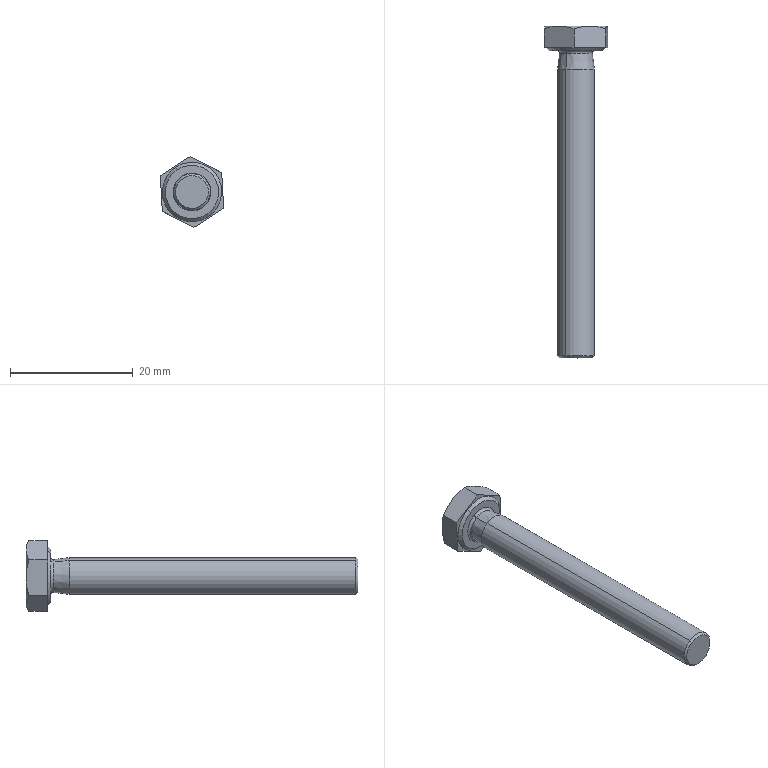Part | STEP file | Cut-Revolve 2-27 | 1 solid | 28 faces | box 10.303 x 54 x 11.529 mm | volume 1738 mm3 | cone 12 | plane 10 | torus 4 | cylinder 2 | commonest cylinder face diameters 6 x2
STEP:
#1=CARTESIAN_POINT('',(-1537.701,1729.714,2771.49));
#2=VERTEX_POINT('',#1);
#3=CARTESIAN_POINT('',(-1537.92,1730.114,2771.825));
#4=VERTEX_POINT('',#3);
#5=CARTESIAN_POINT('',(-1537.92,1729.714,2771.825));
#6=DIRECTION('',(0.8372,0.,0.5469));
#7=DIRECTION('',(0.5469,0.,-0.8372));
#8=AXIS2_PLACEMENT_3D('',#5,#6,#7);
#9=CIRCLE('',#8,0.4);
#10=EDGE_CURVE('',#2,#4,#9,.T.);
#11=ORIENTED_EDGE('',*,*,#10,.F.);
#12=CARTESIAN_POINT('',(-1534.775,1729.714,2767.011));
#13=VERTEX_POINT('',#12);
#14=CARTESIAN_POINT('',(-1536.238,1729.714,2769.251));
#15=DIRECTION('',(0.,1.,0.));
#16=DIRECTION('',(-0.5469,0.,0.8372));
#17=AXIS2_PLACEMENT_3D('',#14,#15,#16);
#18=CIRCLE('',#17,2.675);
#19=EDGE_CURVE('',#2,#13,#18,.T.);
#20=ORIENTED_EDGE('',*,*,#19,.T.);
#21=CARTESIAN_POINT('',(-1534.556,1730.114,2766.676));
#22=VERTEX_POINT('',#21);
#23=CARTESIAN_POINT('',(-1534.556,1729.714,2766.676));
#24=DIRECTION('',(-0.8372,0.,-0.5469));
#25=DIRECTION('',(-0.5469,0.,0.8372));
#26=AXIS2_PLACEMENT_3D('',#23,#24,#25);
#27=CIRCLE('',#26,0.4);
#28=EDGE_CURVE('',#13,#22,#27,.T.);
#29=ORIENTED_EDGE('',*,*,#28,.T.);
#30=CARTESIAN_POINT('',(-1536.238,1730.114,2769.251));
#31=DIRECTION('',(0.,1.,0.));
#32=DIRECTION('',(-0.5469,0.,0.8372));
#33=AXIS2_PLACEMENT_3D('',#30,#31,#32);
#34=CIRCLE('',#33,3.075);
#35=EDGE_CURVE('',#4,#22,#34,.T.);
#36=ORIENTED_EDGE('',*,*,#35,.F.);
#37=EDGE_LOOP('',(#11,#20,#29,#36));
#38=FACE_OUTER_BOUND('',#37,.T.);
#39=CARTESIAN_POINT('',(-1536.238,1729.714,2769.251));
#40=DIRECTION('',(0.,1.,0.));
#41=DIRECTION('',(0.5469,0.,-0.8372));
#42=AXIS2_PLACEMENT_3D('',#39,#40,#41);
#43=TOROIDAL_SURFACE('',#42,3.075,0.4);
#44=ADVANCED_FACE('',(#38),#43,.F.);
#45=ORIENTED_EDGE('',*,*,#28,.F.);
#46=CARTESIAN_POINT('',(-1536.238,1729.714,2769.251));
#47=DIRECTION('',(0.,1.,0.));
#48=DIRECTION('',(-0.5469,0.,0.8372));
#49=AXIS2_PLACEMENT_3D('',#46,#47,#48);
#50=CIRCLE('',#49,2.675);
#51=EDGE_CURVE('',#13,#2,#50,.T.);
#52=ORIENTED_EDGE('',*,*,#51,.T.);
#53=ORIENTED_EDGE('',*,*,#10,.T.);
#54=CARTESIAN_POINT('',(-1536.238,1730.114,2769.251));
#55=DIRECTION('',(0.,1.,0.));
#56=DIRECTION('',(-0.5469,0.,0.8372));
#57=AXIS2_PLACEMENT_3D('',#54,#55,#56);
#58=CIRCLE('',#57,3.075);
#59=EDGE_CURVE('',#22,#4,#58,.T.);
#60=ORIENTED_EDGE('',*,*,#59,.F.);
#61=EDGE_LOOP('',(#45,#52,#53,#60));
#62=FACE_OUTER_BOUND('',#61,.T.);
#63=CARTESIAN_POINT('',(-1536.238,1729.714,2769.251));
#64=DIRECTION('',(0.,1.,0.));
#65=DIRECTION('',(0.5469,0.,-0.8372));
#66=AXIS2_PLACEMENT_3D('',#63,#64,#65);
#67=TOROIDAL_SURFACE('',#66,3.075,0.4);
#68=ADVANCED_FACE('',(#62),#67,.F.);
#69=CARTESIAN_POINT('',(-1538.612,1730.114,2772.884));
#70=VERTEX_POINT('',#69);
#71=CARTESIAN_POINT('',(-1533.865,1730.114,2765.617));
#72=VERTEX_POINT('',#71);
#73=CARTESIAN_POINT('',(-1536.238,1730.114,2769.251));
#74=DIRECTION('',(0.,1.,0.));
#75=DIRECTION('',(-0.5469,0.,0.8372));
#76=AXIS2_PLACEMENT_3D('',#73,#74,#75);
#77=CIRCLE('',#76,4.34);
#78=EDGE_CURVE('',#70,#72,#77,.T.);
#79=ORIENTED_EDGE('',*,*,#78,.T.);
#80=CARTESIAN_POINT('',(-1533.591,1730.614,2765.199));
#81=VERTEX_POINT('',#80);
#82=CARTESIAN_POINT('',(-1533.591,1730.614,2765.199));
#83=DIRECTION('',(0.3867,0.7071,-0.592));
#84=VECTOR('',#83,1000.);
#85=LINE('',#82,#84);
#86=EDGE_CURVE('',#72,#81,#85,.T.);
#87=ORIENTED_EDGE('',*,*,#86,.T.);
#88=CARTESIAN_POINT('',(-1538.885,1730.614,2773.303));
#89=VERTEX_POINT('',#88);
#90=CARTESIAN_POINT('',(-1536.238,1730.614,2769.251));
#91=DIRECTION('',(0.,1.,0.));
#92=DIRECTION('',(-0.5469,0.,0.8372));
#93=AXIS2_PLACEMENT_3D('',#90,#91,#92);
#94=CIRCLE('',#93,4.84);
#95=EDGE_CURVE('',#89,#81,#94,.T.);
#96=ORIENTED_EDGE('',*,*,#95,.F.);
#97=CARTESIAN_POINT('',(-1538.885,1730.614,2773.303));
#98=DIRECTION('',(-0.3867,0.7071,0.592));
#99=VECTOR('',#98,1000.);
#100=LINE('',#97,#99);
#101=EDGE_CURVE('',#70,#89,#100,.T.);
#102=ORIENTED_EDGE('',*,*,#101,.F.);
#103=EDGE_LOOP('',(#79,#87,#96,#102));
#104=FACE_OUTER_BOUND('',#103,.T.);
#105=CARTESIAN_POINT('',(-1536.238,1730.614,2769.251));
#106=DIRECTION('',(0.,1.,0.));
#107=DIRECTION('',(0.5469,0.,-0.8372));
#108=AXIS2_PLACEMENT_3D('',#105,#106,#107);
#109=CONICAL_SURFACE('',#108,4.84,0.7854);
#110=ADVANCED_FACE('',(#104),#109,.T.);
#111=CARTESIAN_POINT('',(-1534.78,1680.114,2767.018));
#112=VERTEX_POINT('',#111);
#113=CARTESIAN_POINT('',(-1537.697,1680.114,2771.483));
#114=VERTEX_POINT('',#113);
#115=CARTESIAN_POINT('',(-1536.238,1680.114,2769.251));
#116=DIRECTION('',(0.,-1.,0.));
#117=DIRECTION('',(-0.5469,0.,0.8372));
#118=AXIS2_PLACEMENT_3D('',#115,#116,#117);
#119=CIRCLE('',#118,2.667);
#120=EDGE_CURVE('',#112,#114,#119,.T.);
#121=ORIENTED_EDGE('',*,*,#120,.F.);
#122=CARTESIAN_POINT('',(-1534.597,1680.448,2766.739));
#123=VERTEX_POINT('',#122);
#124=CARTESIAN_POINT('',(-1534.597,1680.448,2766.739));
#125=DIRECTION('',(0.3867,0.7071,-0.592));
#126=VECTOR('',#125,1000.);
#127=LINE('',#124,#126);
#128=EDGE_CURVE('',#112,#123,#127,.T.);
#129=ORIENTED_EDGE('',*,*,#128,.T.);
#130=CARTESIAN_POINT('',(-1537.879,1680.448,2771.762));
#131=VERTEX_POINT('',#130);
#132=CARTESIAN_POINT('',(-1536.238,1680.448,2769.251));
#133=DIRECTION('',(0.,1.,0.));
#134=DIRECTION('',(-0.5469,0.,0.8372));
#135=AXIS2_PLACEMENT_3D('',#132,#133,#134);
#136=CIRCLE('',#135,3.);
#137=EDGE_CURVE('',#131,#123,#136,.T.);
#138=ORIENTED_EDGE('',*,*,#137,.F.);
#139=CARTESIAN_POINT('',(-1537.879,1680.448,2771.762));
#140=DIRECTION('',(-0.3867,0.7071,0.592));
#141=VECTOR('',#140,1000.);
#142=LINE('',#139,#141);
#143=EDGE_CURVE('',#114,#131,#142,.T.);
#144=ORIENTED_EDGE('',*,*,#143,.F.);
#145=EDGE_LOOP('',(#121,#129,#138,#144));
#146=FACE_OUTER_BOUND('',#145,.T.);
#147=CARTESIAN_POINT('',(-1536.238,1680.448,2769.251));
#148=DIRECTION('',(0.,1.,0.));
#149=DIRECTION('',(0.5469,0.,-0.8372));
#150=AXIS2_PLACEMENT_3D('',#147,#148,#149);
#151=CONICAL_SURFACE('',#150,3.,0.7854);
#152=ADVANCED_FACE('',(#146),#151,.T.);
#153=ORIENTED_EDGE('',*,*,#51,.F.);
#154=CARTESIAN_POINT('',(-1534.773,1729.664,2767.008));
#155=VERTEX_POINT('',#154);
#156=CARTESIAN_POINT('',(-1534.556,1729.714,2766.676));
#157=DIRECTION('',(0.8372,0.,0.5469));
#158=DIRECTION('',(-0.5469,0.,0.8372));
#159=AXIS2_PLACEMENT_3D('',#156,#157,#158);
#160=CIRCLE('',#159,0.4);
#161=EDGE_CURVE('',#13,#155,#160,.T.);
#162=ORIENTED_EDGE('',*,*,#161,.T.);
#163=CARTESIAN_POINT('',(-1537.703,1729.664,2771.493));
#164=VERTEX_POINT('',#163);
#165=CARTESIAN_POINT('',(-1536.238,1729.664,2769.251));
#166=DIRECTION('',(0.,1.,0.));
#167=DIRECTION('',(-0.5469,0.,0.8372));
#168=AXIS2_PLACEMENT_3D('',#165,#166,#167);
#169=CIRCLE('',#168,2.678);
#170=EDGE_CURVE('',#155,#164,#169,.T.);
#171=ORIENTED_EDGE('',*,*,#170,.T.);
#172=CARTESIAN_POINT('',(-1537.92,1729.714,2771.825));
#173=DIRECTION('',(-0.8372,0.,-0.5469));
#174=DIRECTION('',(0.5469,0.,-0.8372));
#175=AXIS2_PLACEMENT_3D('',#172,#173,#174);
#176=CIRCLE('',#175,0.4);
#177=EDGE_CURVE('',#2,#164,#176,.T.);
#178=ORIENTED_EDGE('',*,*,#177,.F.);
#179=EDGE_LOOP('',(#153,#162,#171,#178));
#180=FACE_OUTER_BOUND('',#179,.T.);
#181=CARTESIAN_POINT('',(-1536.238,1729.714,2769.251));
#182=DIRECTION('',(0.,1.,0.));
#183=DIRECTION('',(0.5469,0.,-0.8372));
#184=AXIS2_PLACEMENT_3D('',#181,#182,#183);
#185=TOROIDAL_SURFACE('',#184,3.075,0.4);
#186=ADVANCED_FACE('',(#180),#185,.F.);
#187=ORIENTED_EDGE('',*,*,#137,.T.);
#188=CARTESIAN_POINT('',(-1534.597,1727.114,2766.739));
#189=VERTEX_POINT('',#188);
#190=CARTESIAN_POINT('',(-1534.597,1730.114,2766.739));
#191=DIRECTION('',(0.,1.,0.));
#192=VECTOR('',#191,1000.);
#193=LINE('',#190,#192);
#194=EDGE_CURVE('',#123,#189,#193,.T.);
#195=ORIENTED_EDGE('',*,*,#194,.T.);
#196=CARTESIAN_POINT('',(-1537.879,1727.114,2771.762));
#197=VERTEX_POINT('',#196);
#198=CARTESIAN_POINT('',(-1536.238,1727.114,2769.251));
#199=DIRECTION('',(0.,1.,0.));
#200=DIRECTION('',(-0.5469,0.,0.8372));
#201=AXIS2_PLACEMENT_3D('',#198,#199,#200);
#202=CIRCLE('',#201,3.);
#203=EDGE_CURVE('',#197,#189,#202,.T.);
#204=ORIENTED_EDGE('',*,*,#203,.F.);
#205=CARTESIAN_POINT('',(-1537.879,1730.114,2771.762));
#206=DIRECTION('',(0.,1.,0.));
#207=VECTOR('',#206,1000.);
#208=LINE('',#205,#207);
#209=EDGE_CURVE('',#131,#197,#208,.T.);
#210=ORIENTED_EDGE('',*,*,#209,.F.);
#211=EDGE_LOOP('',(#187,#195,#204,#210));
#212=FACE_OUTER_BOUND('',#211,.T.);
#213=CARTESIAN_POINT('',(-1536.238,1730.114,2769.251));
#214=DIRECTION('',(0.,1.,0.));
#215=DIRECTION('',(0.5469,0.,-0.8372));
#216=AXIS2_PLACEMENT_3D('',#213,#214,#215);
#217=CYLINDRICAL_SURFACE('',#216,3.);
#218=ADVANCED_FACE('',(#212),#217,.T.);
#219=CARTESIAN_POINT('',(-1536.238,1729.664,2769.251));
#220=DIRECTION('',(0.,1.,0.));
#221=DIRECTION('',(-0.5469,0.,0.8372));
#222=AXIS2_PLACEMENT_3D('',#219,#220,#221);
#223=CIRCLE('',#222,2.678);
#224=EDGE_CURVE('',#164,#155,#223,.T.);
#225=ORIENTED_EDGE('',*,*,#224,.F.);
#226=CARTESIAN_POINT('',(-1537.879,1727.114,2771.762));
#227=DIRECTION('',(0.06844,0.9921,-0.1048));
#228=VECTOR('',#227,1000.);
#229=LINE('',#226,#228);
#230=EDGE_CURVE('',#197,#164,#229,.T.);
#231=ORIENTED_EDGE('',*,*,#230,.F.);
#232=ORIENTED_EDGE('',*,*,#203,.T.);
#233=CARTESIAN_POINT('',(-1534.597,1727.114,2766.739));
#234=DIRECTION('',(-0.06844,0.9921,0.1048));
#235=VECTOR('',#234,1000.);
#236=LINE('',#233,#235);
#237=EDGE_CURVE('',#189,#155,#236,.T.);
#238=ORIENTED_EDGE('',*,*,#237,.T.);
#239=EDGE_LOOP('',(#225,#231,#232,#238));
#240=FACE_OUTER_BOUND('',#239,.T.);
#241=CARTESIAN_POINT('',(-1536.238,1727.114,2769.251));
#242=DIRECTION('',(0.,-1.,0.));
#243=DIRECTION('',(-0.5469,0.,0.8372));
#244=AXIS2_PLACEMENT_3D('',#241,#242,#243);
#245=CONICAL_SURFACE('',#244,3.,0.1255);
#246=ADVANCED_FACE('',(#240),#245,.T.);
#247=ORIENTED_EDGE('',*,*,#35,.T.);
#248=ORIENTED_EDGE('',*,*,#59,.T.);
#249=EDGE_LOOP('',(#247,#248));
#250=FACE_BOUND('',#249,.T.);
#251=ORIENTED_EDGE('',*,*,#78,.F.);
#252=CARTESIAN_POINT('',(-1536.238,1730.114,2769.251));
#253=DIRECTION('',(0.,1.,0.));
#254=DIRECTION('',(-0.5469,0.,0.8372));
#255=AXIS2_PLACEMENT_3D('',#252,#253,#254);
#256=CIRCLE('',#255,4.34);
#257=EDGE_CURVE('',#72,#70,#256,.T.);
#258=ORIENTED_EDGE('',*,*,#257,.F.);
#259=EDGE_LOOP('',(#251,#258));
#260=FACE_OUTER_BOUND('',#259,.T.);
#261=CARTESIAN_POINT('',(-1531.087,1730.114,2766.644));
#262=DIRECTION('',(0.,-1.,0.));
#263=DIRECTION('',(-0.5469,0.,0.8372));
#264=AXIS2_PLACEMENT_3D('',#261,#262,#263);
#265=PLANE('',#264);
#266=ADVANCED_FACE('',(#250,#260),#265,.T.);
#267=ORIENTED_EDGE('',*,*,#230,.T.);
#268=ORIENTED_EDGE('',*,*,#170,.F.);
#269=ORIENTED_EDGE('',*,*,#237,.F.);
#270=CARTESIAN_POINT('',(-1536.238,1727.114,2769.251));
#271=DIRECTION('',(0.,1.,0.));
#272=DIRECTION('',(-0.5469,0.,0.8372));
#273=AXIS2_PLACEMENT_3D('',#270,#271,#272);
#274=CIRCLE('',#273,3.);
#275=EDGE_CURVE('',#189,#197,#274,.T.);
#276=ORIENTED_EDGE('',*,*,#275,.T.);
#277=EDGE_LOOP('',(#267,#268,#269,#276));
#278=FACE_OUTER_BOUND('',#277,.T.);
#279=CARTESIAN_POINT('',(-1536.238,1727.114,2769.251));
#280=DIRECTION('',(0.,-1.,0.));
#281=DIRECTION('',(-0.5469,0.,0.8372));
#282=AXIS2_PLACEMENT_3D('',#279,#280,#281);
#283=CONICAL_SURFACE('',#282,3.,0.1255);
#284=ADVANCED_FACE('',(#278),#283,.T.);
#285=ORIENTED_EDGE('',*,*,#194,.F.);
#286=CARTESIAN_POINT('',(-1536.238,1680.448,2769.251));
#287=DIRECTION('',(0.,1.,0.));
#288=DIRECTION('',(-0.5469,0.,0.8372));
#289=AXIS2_PLACEMENT_3D('',#286,#287,#288);
#290=CIRCLE('',#289,3.);
#291=EDGE_CURVE('',#123,#131,#290,.T.);
#292=ORIENTED_EDGE('',*,*,#291,.T.);
#293=ORIENTED_EDGE('',*,*,#209,.T.);
#294=ORIENTED_EDGE('',*,*,#275,.F.);
#295=EDGE_LOOP('',(#285,#292,#293,#294));
#296=FACE_OUTER_BOUND('',#295,.T.);
#297=CARTESIAN_POINT('',(-1536.238,1730.114,2769.251));
#298=DIRECTION('',(0.,1.,0.));
#299=DIRECTION('',(0.5469,0.,-0.8372));
#300=AXIS2_PLACEMENT_3D('',#297,#298,#299);
#301=CYLINDRICAL_SURFACE('',#300,3.);
#302=ADVANCED_FACE('',(#296),#301,.T.);
#303=CARTESIAN_POINT('',(-1536.238,1680.114,2769.251));
#304=DIRECTION('',(0.,-1.,0.));
#305=DIRECTION('',(-0.5469,0.,0.8372));
#306=AXIS2_PLACEMENT_3D('',#303,#304,#305);
#307=CIRCLE('',#306,2.667);
#308=EDGE_CURVE('',#114,#112,#307,.T.);
#309=ORIENTED_EDGE('',*,*,#308,.T.);
#310=ORIENTED_EDGE('',*,*,#120,.T.);
#311=EDGE_LOOP('',(#309,#310));
#312=FACE_OUTER_BOUND('',#311,.T.);
#313=CARTESIAN_POINT('',(-1533.727,1680.114,2770.892));
#314=DIRECTION('',(0.,1.,0.));
#315=DIRECTION('',(0.5469,0.,-0.8372));
#316=AXIS2_PLACEMENT_3D('',#313,#314,#315);
#317=PLANE('',#316);
#318=ADVANCED_FACE('',(#312),#317,.F.);
#319=ORIENTED_EDGE('',*,*,#19,.F.);
#320=ORIENTED_EDGE('',*,*,#177,.T.);
#321=ORIENTED_EDGE('',*,*,#224,.T.);
#322=ORIENTED_EDGE('',*,*,#161,.F.);
#323=EDGE_LOOP('',(#319,#320,#321,#322));
#324=FACE_OUTER_BOUND('',#323,.T.);
#325=CARTESIAN_POINT('',(-1536.238,1729.714,2769.251));
#326=DIRECTION('',(0.,1.,0.));
#327=DIRECTION('',(0.5469,0.,-0.8372));
#328=AXIS2_PLACEMENT_3D('',#325,#326,#327);
#329=TOROIDAL_SURFACE('',#328,3.075,0.4);
#330=ADVANCED_FACE('',(#324),#329,.F.);
#331=ORIENTED_EDGE('',*,*,#128,.F.);
#332=ORIENTED_EDGE('',*,*,#308,.F.);
#333=ORIENTED_EDGE('',*,*,#143,.T.);
#334=ORIENTED_EDGE('',*,*,#291,.F.);
#335=EDGE_LOOP('',(#331,#332,#333,#334));
#336=FACE_OUTER_BOUND('',#335,.T.);
#337=CARTESIAN_POINT('',(-1536.238,1680.448,2769.251));
#338=DIRECTION('',(0.,1.,0.));
#339=DIRECTION('',(0.5469,0.,-0.8372));
#340=AXIS2_PLACEMENT_3D('',#337,#338,#339);
#341=CONICAL_SURFACE('',#340,3.,0.7854);
#342=ADVANCED_FACE('',(#336),#341,.T.);
#343=ORIENTED_EDGE('',*,*,#95,.T.);
#344=CARTESIAN_POINT('',(-1536.238,1730.614,2769.251));
#345=DIRECTION('',(0.,1.,0.));
#346=DIRECTION('',(-0.5469,0.,0.8372));
#347=AXIS2_PLACEMENT_3D('',#344,#345,#346);
#348=CIRCLE('',#347,4.84);
#349=EDGE_CURVE('',#81,#89,#348,.T.);
#350=ORIENTED_EDGE('',*,*,#349,.T.);
#351=EDGE_LOOP('',(#343,#350));
#352=FACE_BOUND('',#351,.T.);
#353=CARTESIAN_POINT('',(-1535.92,1730.614,2763.486));
#354=VERTEX_POINT('',#353);
#355=CARTESIAN_POINT('',(-1531.087,1730.614,2766.644));
#356=VERTEX_POINT('',#355);
#357=CARTESIAN_POINT('',(-1535.92,1730.614,2763.486));
#358=DIRECTION('',(0.8372,0.,0.5469));
#359=VECTOR('',#358,1000.);
#360=LINE('',#357,#359);
#361=EDGE_CURVE('',#354,#356,#360,.T.);
#362=ORIENTED_EDGE('',*,*,#361,.T.);
#363=CARTESIAN_POINT('',(-1531.405,1730.614,2772.408));
#364=VERTEX_POINT('',#363);
#365=CARTESIAN_POINT('',(-1531.087,1730.614,2766.644));
#366=DIRECTION('',(-0.05508,0.,0.9985));
#367=VECTOR('',#366,1000.);
#368=LINE('',#365,#367);
#369=EDGE_CURVE('',#356,#364,#368,.T.);
#370=ORIENTED_EDGE('',*,*,#369,.T.);
#371=CARTESIAN_POINT('',(-1536.556,1730.614,2775.015));
#372=VERTEX_POINT('',#371);
#373=CARTESIAN_POINT('',(-1531.405,1730.614,2772.408));
#374=DIRECTION('',(-0.8923,0.,0.4515));
#375=VECTOR('',#374,1000.);
#376=LINE('',#373,#375);
#377=EDGE_CURVE('',#364,#372,#376,.T.);
#378=ORIENTED_EDGE('',*,*,#377,.T.);
#379=CARTESIAN_POINT('',(-1541.39,1730.614,2771.858));
#380=VERTEX_POINT('',#379);
#381=CARTESIAN_POINT('',(-1536.556,1730.614,2775.015));
#382=DIRECTION('',(-0.8372,0.,-0.5469));
#383=VECTOR('',#382,1000.);
#384=LINE('',#381,#383);
#385=EDGE_CURVE('',#372,#380,#384,.T.);
#386=ORIENTED_EDGE('',*,*,#385,.T.);
#387=CARTESIAN_POINT('',(-1541.072,1730.614,2766.093));
#388=VERTEX_POINT('',#387);
#389=CARTESIAN_POINT('',(-1541.39,1730.614,2771.858));
#390=DIRECTION('',(0.05508,0.,-0.9985));
#391=VECTOR('',#390,1000.);
#392=LINE('',#389,#391);
#393=EDGE_CURVE('',#380,#388,#392,.T.);
#394=ORIENTED_EDGE('',*,*,#393,.T.);
#395=CARTESIAN_POINT('',(-1541.072,1730.614,2766.093));
#396=DIRECTION('',(0.8923,0.,-0.4515));
#397=VECTOR('',#396,1000.);
#398=LINE('',#395,#397);
#399=EDGE_CURVE('',#388,#354,#398,.T.);
#400=ORIENTED_EDGE('',*,*,#399,.T.);
#401=EDGE_LOOP('',(#362,#370,#378,#386,#394,#400));
#402=FACE_OUTER_BOUND('',#401,.T.);
#403=CARTESIAN_POINT('',(-1540.29,1730.614,2766.603));
#404=DIRECTION('',(0.,-1.,0.));
#405=DIRECTION('',(-0.5469,0.,0.8372));
#406=AXIS2_PLACEMENT_3D('',#403,#404,#405);
#407=PLANE('',#406);
#408=ADVANCED_FACE('',(#352,#402),#407,.T.);
#409=ORIENTED_EDGE('',*,*,#86,.F.);
#410=ORIENTED_EDGE('',*,*,#257,.T.);
#411=ORIENTED_EDGE('',*,*,#101,.T.);
#412=ORIENTED_EDGE('',*,*,#349,.F.);
#413=EDGE_LOOP('',(#409,#410,#411,#412));
#414=FACE_OUTER_BOUND('',#413,.T.);
#415=CARTESIAN_POINT('',(-1536.238,1730.614,2769.251));
#416=DIRECTION('',(0.,1.,0.));
#417=DIRECTION('',(0.5469,0.,-0.8372));
#418=AXIS2_PLACEMENT_3D('',#415,#416,#417);
#419=CONICAL_SURFACE('',#418,4.84,0.7854);
#420=ADVANCED_FACE('',(#414),#419,.T.);
#421=CARTESIAN_POINT('',(-1533.504,1734.114,2765.065));
#422=VERTEX_POINT('',#421);
#423=CARTESIAN_POINT('',(-1531.246,1734.114,2769.526));
#424=VERTEX_POINT('',#423);
#425=CARTESIAN_POINT('',(-1536.238,1734.114,2769.251));
#426=DIRECTION('',(0.,-1.,0.));
#427=DIRECTION('',(0.5469,0.,-0.8372));
#428=AXIS2_PLACEMENT_3D('',#425,#426,#427);
#429=CIRCLE('',#428,5.);
#430=EDGE_CURVE('',#422,#424,#429,.T.);
#431=ORIENTED_EDGE('',*,*,#430,.F.);
#432=CARTESIAN_POINT('',(-1538.496,1734.114,2764.789));
#433=VERTEX_POINT('',#432);
#434=CARTESIAN_POINT('',(-1536.238,1734.114,2769.251));
#435=DIRECTION('',(0.,-1.,0.));
#436=DIRECTION('',(0.5469,0.,-0.8372));
#437=AXIS2_PLACEMENT_3D('',#434,#435,#436);
#438=CIRCLE('',#437,5.);
#439=EDGE_CURVE('',#433,#422,#438,.T.);
#440=ORIENTED_EDGE('',*,*,#439,.F.);
#441=CARTESIAN_POINT('',(-1541.231,1734.114,2768.975));
#442=VERTEX_POINT('',#441);
#443=CARTESIAN_POINT('',(-1536.238,1734.114,2769.251));
#444=DIRECTION('',(0.,-1.,0.));
#445=DIRECTION('',(0.5469,0.,-0.8372));
#446=AXIS2_PLACEMENT_3D('',#443,#444,#445);
#447=CIRCLE('',#446,5.);
#448=EDGE_CURVE('',#442,#433,#447,.T.);
#449=ORIENTED_EDGE('',*,*,#448,.F.);
#450=CARTESIAN_POINT('',(-1538.973,1734.114,2773.437));
#451=VERTEX_POINT('',#450);
#452=CARTESIAN_POINT('',(-1536.238,1734.114,2769.251));
#453=DIRECTION('',(0.,-1.,0.));
#454=DIRECTION('',(0.5469,0.,-0.8372));
#455=AXIS2_PLACEMENT_3D('',#452,#453,#454);
#456=CIRCLE('',#455,5.);
#457=EDGE_CURVE('',#451,#442,#456,.T.);
#458=ORIENTED_EDGE('',*,*,#457,.F.);
#459=CARTESIAN_POINT('',(-1533.981,1734.114,2773.712));
#460=VERTEX_POINT('',#459);
#461=CARTESIAN_POINT('',(-1536.238,1734.114,2769.251));
#462=DIRECTION('',(0.,1.,0.));
#463=DIRECTION('',(-0.5469,0.,0.8372));
#464=AXIS2_PLACEMENT_3D('',#461,#462,#463);
#465=CIRCLE('',#464,5.);
#466=EDGE_CURVE('',#451,#460,#465,.T.);
#467=ORIENTED_EDGE('',*,*,#466,.T.);
#468=CARTESIAN_POINT('',(-1536.238,1734.114,2769.251));
#469=DIRECTION('',(0.,-1.,0.));
#470=DIRECTION('',(0.5469,0.,-0.8372));
#471=AXIS2_PLACEMENT_3D('',#468,#469,#470);
#472=CIRCLE('',#471,5.);
#473=EDGE_CURVE('',#424,#460,#472,.T.);
#474=ORIENTED_EDGE('',*,*,#473,.F.);
#475=EDGE_LOOP('',(#431,#440,#449,#458,#467,#474));
#476=FACE_OUTER_BOUND('',#475,.T.);
#477=CARTESIAN_POINT('',(-1531.087,1734.114,2766.644));
#478=DIRECTION('',(0.,-1.,0.));
#479=DIRECTION('',(-0.5469,0.,0.8372));
#480=AXIS2_PLACEMENT_3D('',#477,#478,#479);
#481=PLANE('',#480);
#482=ADVANCED_FACE('',(#476),#481,.F.);
#483=CARTESIAN_POINT('',(-1531.087,1733.668,2766.644));
#484=VERTEX_POINT('',#483);
#485=CARTESIAN_POINT('',(-1531.246,1734.114,2769.526));
#486=CARTESIAN_POINT('',(-1531.192,1734.114,2768.542));
#487=CARTESIAN_POINT('',(-1531.139,1733.94,2767.585));
#488=CARTESIAN_POINT('',(-1531.087,1733.668,2766.644));
#489=B_SPLINE_CURVE_WITH_KNOTS('',3,(#485,#486,#487,#488),.UNSPECIFIED.,.F.,.F.,(4,4),(0.,0.002921),.UNSPECIFIED.);
#490=EDGE_CURVE('',#424,#484,#489,.T.);
#491=ORIENTED_EDGE('',*,*,#490,.T.);
#492=CARTESIAN_POINT('',(-1531.087,1733.668,2766.644));
#493=CARTESIAN_POINT('',(-1531.876,1733.94,2766.128));
#494=CARTESIAN_POINT('',(-1532.679,1734.114,2765.604));
#495=CARTESIAN_POINT('',(-1533.504,1734.114,2765.065));
#496=B_SPLINE_CURVE_WITH_KNOTS('',3,(#492,#493,#494,#495),.UNSPECIFIED.,.F.,.F.,(4,4),(0.,0.002921),.UNSPECIFIED.);
#497=EDGE_CURVE('',#484,#422,#496,.T.);
#498=ORIENTED_EDGE('',*,*,#497,.T.);
#499=ORIENTED_EDGE('',*,*,#430,.T.);
#500=EDGE_LOOP('',(#491,#498,#499));
#501=FACE_OUTER_BOUND('',#500,.T.);
#502=CARTESIAN_POINT('',(-1536.238,1734.114,2769.251));
#503=DIRECTION('',(0.,-1.,0.));
#504=DIRECTION('',(0.5469,0.,-0.8372));
#505=AXIS2_PLACEMENT_3D('',#502,#503,#504);
#506=CONICAL_SURFACE('',#505,5.,1.047);
#507=ADVANCED_FACE('',(#501),#506,.T.);
#508=CARTESIAN_POINT('',(-1531.405,1733.668,2772.408));
#509=VERTEX_POINT('',#508);
#510=CARTESIAN_POINT('',(-1533.981,1734.114,2773.712));
#511=CARTESIAN_POINT('',(-1533.101,1734.114,2773.267));
#512=CARTESIAN_POINT('',(-1532.246,1733.94,2772.834));
#513=CARTESIAN_POINT('',(-1531.405,1733.668,2772.408));
#514=B_SPLINE_CURVE_WITH_KNOTS('',3,(#510,#511,#512,#513),.UNSPECIFIED.,.F.,.F.,(4,4),(0.,0.002921),.UNSPECIFIED.);
#515=EDGE_CURVE('',#460,#509,#514,.T.);
#516=ORIENTED_EDGE('',*,*,#515,.T.);
#517=CARTESIAN_POINT('',(-1531.405,1733.668,2772.408));
#518=CARTESIAN_POINT('',(-1531.353,1733.94,2771.467));
#519=CARTESIAN_POINT('',(-1531.3,1734.114,2770.51));
#520=CARTESIAN_POINT('',(-1531.246,1734.114,2769.526));
#521=B_SPLINE_CURVE_WITH_KNOTS('',3,(#517,#518,#519,#520),.UNSPECIFIED.,.F.,.F.,(4,4),(0.,0.002921),.UNSPECIFIED.);
#522=EDGE_CURVE('',#509,#424,#521,.T.);
#523=ORIENTED_EDGE('',*,*,#522,.T.);
#524=ORIENTED_EDGE('',*,*,#473,.T.);
#525=EDGE_LOOP('',(#516,#523,#524));
#526=FACE_OUTER_BOUND('',#525,.T.);
#527=CARTESIAN_POINT('',(-1536.238,1734.114,2769.251));
#528=DIRECTION('',(0.,-1.,0.));
#529=DIRECTION('',(0.5469,0.,-0.8372));
#530=AXIS2_PLACEMENT_3D('',#527,#528,#529);
#531=CONICAL_SURFACE('',#530,5.,1.047);
#532=ADVANCED_FACE('',(#526),#531,.T.);
#533=CARTESIAN_POINT('',(-1536.556,1733.668,2775.015));
#534=VERTEX_POINT('',#533);
#535=CARTESIAN_POINT('',(-1536.556,1733.668,2775.015));
#536=CARTESIAN_POINT('',(-1535.715,1733.94,2774.59));
#537=CARTESIAN_POINT('',(-1534.86,1734.114,2774.157));
#538=CARTESIAN_POINT('',(-1533.981,1734.114,2773.712));
#539=B_SPLINE_CURVE_WITH_KNOTS('',3,(#535,#536,#537,#538),.UNSPECIFIED.,.F.,.F.,(4,4),(0.,0.002921),.UNSPECIFIED.);
#540=EDGE_CURVE('',#534,#460,#539,.T.);
#541=ORIENTED_EDGE('',*,*,#540,.T.);
#542=ORIENTED_EDGE('',*,*,#466,.F.);
#543=CARTESIAN_POINT('',(-1538.973,1734.114,2773.437));
#544=CARTESIAN_POINT('',(-1538.148,1734.114,2773.975));
#545=CARTESIAN_POINT('',(-1537.346,1733.94,2774.5));
#546=CARTESIAN_POINT('',(-1536.556,1733.668,2775.015));
#547=B_SPLINE_CURVE_WITH_KNOTS('',3,(#543,#544,#545,#546),.UNSPECIFIED.,.F.,.F.,(4,4),(0.,0.002921),.UNSPECIFIED.);
#548=EDGE_CURVE('',#451,#534,#547,.T.);
#549=ORIENTED_EDGE('',*,*,#548,.T.);
#550=EDGE_LOOP('',(#541,#542,#549));
#551=FACE_OUTER_BOUND('',#550,.T.);
#552=CARTESIAN_POINT('',(-1536.238,1734.114,2769.251));
#553=DIRECTION('',(0.,-1.,0.));
#554=DIRECTION('',(0.5469,0.,-0.8372));
#555=AXIS2_PLACEMENT_3D('',#552,#553,#554);
#556=CONICAL_SURFACE('',#555,5.,1.047);
#557=ADVANCED_FACE('',(#551),#556,.T.);
#558=CARTESIAN_POINT('',(-1541.39,1733.668,2771.858));
#559=VERTEX_POINT('',#558);
#560=CARTESIAN_POINT('',(-1541.39,1733.668,2771.858));
#561=CARTESIAN_POINT('',(-1540.6,1733.94,2772.374));
#562=CARTESIAN_POINT('',(-1539.798,1734.114,2772.898));
#563=CARTESIAN_POINT('',(-1538.973,1734.114,2773.437));
#564=B_SPLINE_CURVE_WITH_KNOTS('',3,(#560,#561,#562,#563),.UNSPECIFIED.,.F.,.F.,(4,4),(0.,0.002921),.UNSPECIFIED.);
#565=EDGE_CURVE('',#559,#451,#564,.T.);
#566=ORIENTED_EDGE('',*,*,#565,.T.);
#567=ORIENTED_EDGE('',*,*,#457,.T.);
#568=CARTESIAN_POINT('',(-1541.231,1734.114,2768.975));
#569=CARTESIAN_POINT('',(-1541.285,1734.114,2769.959));
#570=CARTESIAN_POINT('',(-1541.338,1733.94,2770.916));
#571=CARTESIAN_POINT('',(-1541.39,1733.668,2771.858));
#572=B_SPLINE_CURVE_WITH_KNOTS('',3,(#568,#569,#570,#571),.UNSPECIFIED.,.F.,.F.,(4,4),(0.,0.002921),.UNSPECIFIED.);
#573=EDGE_CURVE('',#442,#559,#572,.T.);
#574=ORIENTED_EDGE('',*,*,#573,.T.);
#575=EDGE_LOOP('',(#566,#567,#574));
#576=FACE_OUTER_BOUND('',#575,.T.);
#577=CARTESIAN_POINT('',(-1536.238,1734.114,2769.251));
#578=DIRECTION('',(0.,-1.,0.));
#579=DIRECTION('',(0.5469,0.,-0.8372));
#580=AXIS2_PLACEMENT_3D('',#577,#578,#579);
#581=CONICAL_SURFACE('',#580,5.,1.047);
#582=ADVANCED_FACE('',(#576),#581,.T.);
#583=CARTESIAN_POINT('',(-1535.92,1733.668,2763.486));
#584=VERTEX_POINT('',#583);
#585=CARTESIAN_POINT('',(-1533.504,1734.114,2765.065));
#586=CARTESIAN_POINT('',(-1534.328,1734.114,2764.526));
#587=CARTESIAN_POINT('',(-1535.131,1733.94,2764.002));
#588=CARTESIAN_POINT('',(-1535.92,1733.668,2763.486));
#589=B_SPLINE_CURVE_WITH_KNOTS('',3,(#585,#586,#587,#588),.UNSPECIFIED.,.F.,.F.,(4,4),(0.,0.002921),.UNSPECIFIED.);
#590=EDGE_CURVE('',#422,#584,#589,.T.);
#591=ORIENTED_EDGE('',*,*,#590,.T.);
#592=CARTESIAN_POINT('',(-1535.92,1733.668,2763.486));
#593=CARTESIAN_POINT('',(-1536.762,1733.94,2763.912));
#594=CARTESIAN_POINT('',(-1537.617,1734.114,2764.345));
#595=CARTESIAN_POINT('',(-1538.496,1734.114,2764.789));
#596=B_SPLINE_CURVE_WITH_KNOTS('',3,(#592,#593,#594,#595),.UNSPECIFIED.,.F.,.F.,(4,4),(0.,0.002921),.UNSPECIFIED.);
#597=EDGE_CURVE('',#584,#433,#596,.T.);
#598=ORIENTED_EDGE('',*,*,#597,.T.);
#599=ORIENTED_EDGE('',*,*,#439,.T.);
#600=EDGE_LOOP('',(#591,#598,#599));
#601=FACE_OUTER_BOUND('',#600,.T.);
#602=CARTESIAN_POINT('',(-1536.238,1734.114,2769.251));
#603=DIRECTION('',(0.,-1.,0.));
#604=DIRECTION('',(0.5469,0.,-0.8372));
#605=AXIS2_PLACEMENT_3D('',#602,#603,#604);
#606=CONICAL_SURFACE('',#605,5.,1.047);
#607=ADVANCED_FACE('',(#601),#606,.T.);
#608=CARTESIAN_POINT('',(-1541.072,1733.668,2766.093));
#609=VERTEX_POINT('',#608);
#610=CARTESIAN_POINT('',(-1541.072,1733.668,2766.093));
#611=CARTESIAN_POINT('',(-1541.124,1733.94,2767.035));
#612=CARTESIAN_POINT('',(-1541.176,1734.114,2767.992));
#613=CARTESIAN_POINT('',(-1541.231,1734.114,2768.975));
#614=B_SPLINE_CURVE_WITH_KNOTS('',3,(#610,#611,#612,#613),.UNSPECIFIED.,.F.,.F.,(4,4),(0.,0.002921),.UNSPECIFIED.);
#615=EDGE_CURVE('',#609,#442,#614,.T.);
#616=ORIENTED_EDGE('',*,*,#615,.T.);
#617=ORIENTED_EDGE('',*,*,#448,.T.);
#618=CARTESIAN_POINT('',(-1538.496,1734.114,2764.789));
#619=CARTESIAN_POINT('',(-1539.375,1734.114,2765.234));
#620=CARTESIAN_POINT('',(-1540.23,1733.94,2765.667));
#621=CARTESIAN_POINT('',(-1541.072,1733.668,2766.093));
#622=B_SPLINE_CURVE_WITH_KNOTS('',3,(#618,#619,#620,#621),.UNSPECIFIED.,.F.,.F.,(4,4),(0.,0.002921),.UNSPECIFIED.);
#623=EDGE_CURVE('',#433,#609,#622,.T.);
#624=ORIENTED_EDGE('',*,*,#623,.T.);
#625=EDGE_LOOP('',(#616,#617,#624));
#626=FACE_OUTER_BOUND('',#625,.T.);
#627=CARTESIAN_POINT('',(-1536.238,1734.114,2769.251));
#628=DIRECTION('',(0.,-1.,0.));
#629=DIRECTION('',(0.5469,0.,-0.8372));
#630=AXIS2_PLACEMENT_3D('',#627,#628,#629);
#631=CONICAL_SURFACE('',#630,5.,1.047);
#632=ADVANCED_FACE('',(#626),#631,.T.);
#633=ORIENTED_EDGE('',*,*,#399,.F.);
#634=CARTESIAN_POINT('',(-1541.072,1730.114,2766.093));
#635=DIRECTION('',(0.,1.,0.));
#636=VECTOR('',#635,1000.);
#637=LINE('',#634,#636);
#638=EDGE_CURVE('',#388,#609,#637,.T.);
#639=ORIENTED_EDGE('',*,*,#638,.T.);
#640=ORIENTED_EDGE('',*,*,#623,.F.);
#641=ORIENTED_EDGE('',*,*,#597,.F.);
#642=CARTESIAN_POINT('',(-1535.92,1730.114,2763.486));
#643=DIRECTION('',(0.,1.,0.));
#644=VECTOR('',#643,1000.);
#645=LINE('',#642,#644);
#646=EDGE_CURVE('',#354,#584,#645,.T.);
#647=ORIENTED_EDGE('',*,*,#646,.F.);
#648=EDGE_LOOP('',(#633,#639,#640,#641,#647));
#649=FACE_OUTER_BOUND('',#648,.T.);
#650=CARTESIAN_POINT('',(-1541.072,1730.114,2766.093));
#651=DIRECTION('',(0.4515,0.,0.8923));
#652=DIRECTION('',(0.8923,0.,-0.4515));
#653=AXIS2_PLACEMENT_3D('',#650,#651,#652);
#654=PLANE('',#653);
#655=ADVANCED_FACE('',(#649),#654,.F.);
#656=ORIENTED_EDGE('',*,*,#393,.F.);
#657=CARTESIAN_POINT('',(-1541.39,1730.114,2771.858));
#658=DIRECTION('',(0.,1.,0.));
#659=VECTOR('',#658,1000.);
#660=LINE('',#657,#659);
#661=EDGE_CURVE('',#380,#559,#660,.T.);
#662=ORIENTED_EDGE('',*,*,#661,.T.);
#663=ORIENTED_EDGE('',*,*,#573,.F.);
#664=ORIENTED_EDGE('',*,*,#615,.F.);
#665=ORIENTED_EDGE('',*,*,#638,.F.);
#666=EDGE_LOOP('',(#656,#662,#663,#664,#665));
#667=FACE_OUTER_BOUND('',#666,.T.);
#668=CARTESIAN_POINT('',(-1541.39,1730.114,2771.858));
#669=DIRECTION('',(0.9985,0.,0.05508));
#670=DIRECTION('',(0.05508,0.,-0.9985));
#671=AXIS2_PLACEMENT_3D('',#668,#669,#670);
#672=PLANE('',#671);
#673=ADVANCED_FACE('',(#667),#672,.F.);
#674=ORIENTED_EDGE('',*,*,#385,.F.);
#675=CARTESIAN_POINT('',(-1536.556,1730.114,2775.015));
#676=DIRECTION('',(0.,1.,0.));
#677=VECTOR('',#676,1000.);
#678=LINE('',#675,#677);
#679=EDGE_CURVE('',#372,#534,#678,.T.);
#680=ORIENTED_EDGE('',*,*,#679,.T.);
#681=ORIENTED_EDGE('',*,*,#548,.F.);
#682=ORIENTED_EDGE('',*,*,#565,.F.);
#683=ORIENTED_EDGE('',*,*,#661,.F.);
#684=EDGE_LOOP('',(#674,#680,#681,#682,#683));
#685=FACE_OUTER_BOUND('',#684,.T.);
#686=CARTESIAN_POINT('',(-1536.556,1730.114,2775.015));
#687=DIRECTION('',(0.5469,0.,-0.8372));
#688=DIRECTION('',(0.,-1.,0.));
#689=AXIS2_PLACEMENT_3D('',#686,#687,#688);
#690=PLANE('',#689);
#691=ADVANCED_FACE('',(#685),#690,.F.);
#692=ORIENTED_EDGE('',*,*,#377,.F.);
#693=CARTESIAN_POINT('',(-1531.405,1730.114,2772.408));
#694=DIRECTION('',(0.,1.,0.));
#695=VECTOR('',#694,1000.);
#696=LINE('',#693,#695);
#697=EDGE_CURVE('',#364,#509,#696,.T.);
#698=ORIENTED_EDGE('',*,*,#697,.T.);
#699=ORIENTED_EDGE('',*,*,#515,.F.);
#700=ORIENTED_EDGE('',*,*,#540,.F.);
#701=ORIENTED_EDGE('',*,*,#679,.F.);
#702=EDGE_LOOP('',(#692,#698,#699,#700,#701));
#703=FACE_OUTER_BOUND('',#702,.T.);
#704=CARTESIAN_POINT('',(-1531.405,1730.114,2772.408));
#705=DIRECTION('',(-0.4515,0.,-0.8923));
#706=DIRECTION('',(-0.8923,0.,0.4515));
#707=AXIS2_PLACEMENT_3D('',#704,#705,#706);
#708=PLANE('',#707);
#709=ADVANCED_FACE('',(#703),#708,.F.);
#710=ORIENTED_EDGE('',*,*,#369,.F.);
#711=CARTESIAN_POINT('',(-1531.087,1730.114,2766.644));
#712=DIRECTION('',(0.,1.,0.));
#713=VECTOR('',#712,1000.);
#714=LINE('',#711,#713);
#715=EDGE_CURVE('',#356,#484,#714,.T.);
#716=ORIENTED_EDGE('',*,*,#715,.T.);
#717=ORIENTED_EDGE('',*,*,#490,.F.);
#718=ORIENTED_EDGE('',*,*,#522,.F.);
#719=ORIENTED_EDGE('',*,*,#697,.F.);
#720=EDGE_LOOP('',(#710,#716,#717,#718,#719));
#721=FACE_OUTER_BOUND('',#720,.T.);
#722=CARTESIAN_POINT('',(-1531.087,1730.114,2766.644));
#723=DIRECTION('',(-0.9985,0.,-0.05508));
#724=DIRECTION('',(-0.05508,0.,0.9985));
#725=AXIS2_PLACEMENT_3D('',#722,#723,#724);
#726=PLANE('',#725);
#727=ADVANCED_FACE('',(#721),#726,.F.);
#728=ORIENTED_EDGE('',*,*,#361,.F.);
#729=ORIENTED_EDGE('',*,*,#646,.T.);
#730=ORIENTED_EDGE('',*,*,#590,.F.);
#731=ORIENTED_EDGE('',*,*,#497,.F.);
#732=ORIENTED_EDGE('',*,*,#715,.F.);
#733=EDGE_LOOP('',(#728,#729,#730,#731,#732));
#734=FACE_OUTER_BOUND('',#733,.T.);
#735=CARTESIAN_POINT('',(-1535.92,1730.114,2763.486));
#736=DIRECTION('',(-0.5469,0.,0.8372));
#737=DIRECTION('',(0.8372,0.,0.5469));
#738=AXIS2_PLACEMENT_3D('',#735,#736,#737);
#739=PLANE('',#738);
#740=ADVANCED_FACE('',(#734),#739,.F.);
#741=CLOSED_SHELL('',(#44,#68,#110,#152,#186,#218,#246,#266,#284,#302,#318,#330,#342,#408,#420,#482,#507,#532,#557,#582,#607,#632,#655,#673,#691,#709,#727,#740));
#742=MANIFOLD_SOLID_BREP('',#741);
#743=CARTESIAN_POINT('',(0.,0.,0.));
#744=DIRECTION('',(0.,0.,1.));
#745=DIRECTION('',(1.,0.,0.));
#746=AXIS2_PLACEMENT_3D('',#743,#744,#745);
#747=(LENGTH_UNIT()NAMED_UNIT(*)SI_UNIT(.MILLI.,.METRE.));
#748=UNCERTAINTY_MEASURE_WITH_UNIT(LENGTH_MEASURE(0.00001),#747,'','');
#749=(NAMED_UNIT(*)PLANE_ANGLE_UNIT()SI_UNIT($,.RADIAN.));
#750=(NAMED_UNIT(*)SI_UNIT($,.STERADIAN.)SOLID_ANGLE_UNIT());
#751=(GEOMETRIC_REPRESENTATION_CONTEXT(3)GLOBAL_UNCERTAINTY_ASSIGNED_CONTEXT((#748))GLOBAL_UNIT_ASSIGNED_CONTEXT((#747,#749,#750))REPRESENTATION_CONTEXT('',''));
#752=ADVANCED_BREP_SHAPE_REPRESENTATION('',(#742,#746),#751);